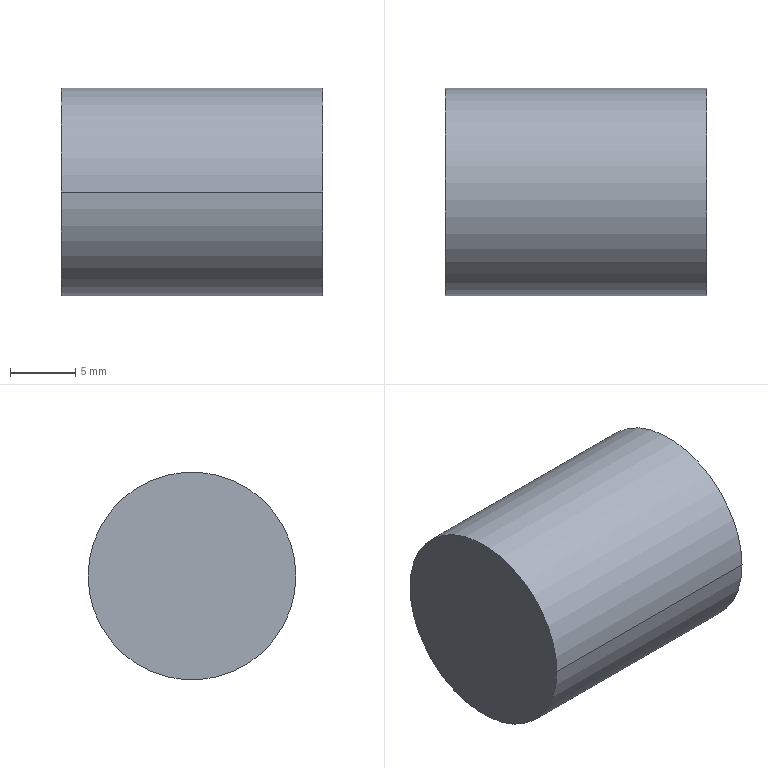Part | STEP file | 4-20.sldasm-Part-191 | 1 solid | 4 faces | box 20 x 15.87 x 15.87 mm | volume 3956 mm3 | cylinder 2 | plane 2 | commonest cylinder face diameters 15.87 x2
STEP:
#1=CARTESIAN_POINT('',(-213.37,-566.51,-38.));
#2=VERTEX_POINT('',#1);
#3=CARTESIAN_POINT('',(-213.37,-550.64,-38.));
#4=VERTEX_POINT('',#3);
#5=CARTESIAN_POINT('',(-213.37,-558.575,-38.));
#6=DIRECTION('',(1.,0.,0.));
#7=DIRECTION('',(0.,1.,0.));
#8=AXIS2_PLACEMENT_3D('',#5,#6,#7);
#9=CIRCLE('',#8,7.935);
#10=EDGE_CURVE('',#2,#4,#9,.T.);
#11=ORIENTED_EDGE('',*,*,#10,.T.);
#12=CARTESIAN_POINT('',(-193.37,-550.64,-38.));
#13=VERTEX_POINT('',#12);
#14=CARTESIAN_POINT('',(-203.37,-550.64,-38.));
#15=DIRECTION('',(1.,0.,0.));
#16=VECTOR('',#15,1000.);
#17=LINE('',#14,#16);
#18=EDGE_CURVE('',#4,#13,#17,.T.);
#19=ORIENTED_EDGE('',*,*,#18,.T.);
#20=CARTESIAN_POINT('',(-193.37,-566.51,-38.));
#21=VERTEX_POINT('',#20);
#22=CARTESIAN_POINT('',(-193.37,-558.575,-38.));
#23=DIRECTION('',(-1.,0.,0.));
#24=DIRECTION('',(0.,-1.,0.));
#25=AXIS2_PLACEMENT_3D('',#22,#23,#24);
#26=CIRCLE('',#25,7.935);
#27=EDGE_CURVE('',#13,#21,#26,.T.);
#28=ORIENTED_EDGE('',*,*,#27,.T.);
#29=CARTESIAN_POINT('',(-203.37,-566.51,-38.));
#30=DIRECTION('',(1.,0.,0.));
#31=VECTOR('',#30,1000.);
#32=LINE('',#29,#31);
#33=EDGE_CURVE('',#2,#21,#32,.T.);
#34=ORIENTED_EDGE('',*,*,#33,.F.);
#35=EDGE_LOOP('',(#11,#19,#28,#34));
#36=FACE_OUTER_BOUND('',#35,.T.);
#37=CARTESIAN_POINT('',(-203.37,-558.575,-38.));
#38=DIRECTION('',(1.,0.,0.));
#39=DIRECTION('',(0.,-1.,0.));
#40=AXIS2_PLACEMENT_3D('',#37,#38,#39);
#41=CYLINDRICAL_SURFACE('',#40,7.935);
#42=ADVANCED_FACE('',(#36),#41,.T.);
#43=CARTESIAN_POINT('',(-193.37,-558.575,-38.));
#44=DIRECTION('',(-1.,0.,0.));
#45=DIRECTION('',(0.,-1.,0.));
#46=AXIS2_PLACEMENT_3D('',#43,#44,#45);
#47=CIRCLE('',#46,7.935);
#48=EDGE_CURVE('',#21,#13,#47,.T.);
#49=ORIENTED_EDGE('',*,*,#48,.F.);
#50=ORIENTED_EDGE('',*,*,#27,.F.);
#51=EDGE_LOOP('',(#49,#50));
#52=FACE_OUTER_BOUND('',#51,.T.);
#53=CARTESIAN_POINT('',(-193.37,-558.575,-38.));
#54=DIRECTION('',(1.,0.,0.));
#55=DIRECTION('',(0.,-1.,0.));
#56=AXIS2_PLACEMENT_3D('',#53,#54,#55);
#57=PLANE('',#56);
#58=ADVANCED_FACE('',(#52),#57,.T.);
#59=ORIENTED_EDGE('',*,*,#10,.F.);
#60=CARTESIAN_POINT('',(-213.37,-558.575,-38.));
#61=DIRECTION('',(1.,0.,0.));
#62=DIRECTION('',(0.,1.,0.));
#63=AXIS2_PLACEMENT_3D('',#60,#61,#62);
#64=CIRCLE('',#63,7.935);
#65=EDGE_CURVE('',#4,#2,#64,.T.);
#66=ORIENTED_EDGE('',*,*,#65,.F.);
#67=EDGE_LOOP('',(#59,#66));
#68=FACE_OUTER_BOUND('',#67,.T.);
#69=CARTESIAN_POINT('',(-213.37,-558.575,-38.));
#70=DIRECTION('',(-1.,0.,0.));
#71=DIRECTION('',(0.,1.,0.));
#72=AXIS2_PLACEMENT_3D('',#69,#70,#71);
#73=PLANE('',#72);
#74=ADVANCED_FACE('',(#68),#73,.T.);
#75=ORIENTED_EDGE('',*,*,#18,.F.);
#76=ORIENTED_EDGE('',*,*,#65,.T.);
#77=ORIENTED_EDGE('',*,*,#33,.T.);
#78=ORIENTED_EDGE('',*,*,#48,.T.);
#79=EDGE_LOOP('',(#75,#76,#77,#78));
#80=FACE_OUTER_BOUND('',#79,.T.);
#81=CARTESIAN_POINT('',(-203.37,-558.575,-38.));
#82=DIRECTION('',(1.,0.,0.));
#83=DIRECTION('',(0.,-1.,0.));
#84=AXIS2_PLACEMENT_3D('',#81,#82,#83);
#85=CYLINDRICAL_SURFACE('',#84,7.935);
#86=ADVANCED_FACE('',(#80),#85,.T.);
#87=CLOSED_SHELL('',(#42,#58,#74,#86));
#88=MANIFOLD_SOLID_BREP('',#87);
#89=CARTESIAN_POINT('',(0.,0.,0.));
#90=DIRECTION('',(0.,0.,1.));
#91=DIRECTION('',(1.,0.,0.));
#92=AXIS2_PLACEMENT_3D('',#89,#90,#91);
#93=(LENGTH_UNIT()NAMED_UNIT(*)SI_UNIT(.MILLI.,.METRE.));
#94=UNCERTAINTY_MEASURE_WITH_UNIT(LENGTH_MEASURE(0.00001),#93,'','');
#95=(NAMED_UNIT(*)PLANE_ANGLE_UNIT()SI_UNIT($,.RADIAN.));
#96=(NAMED_UNIT(*)SI_UNIT($,.STERADIAN.)SOLID_ANGLE_UNIT());
#97=(GEOMETRIC_REPRESENTATION_CONTEXT(3)GLOBAL_UNCERTAINTY_ASSIGNED_CONTEXT((#94))GLOBAL_UNIT_ASSIGNED_CONTEXT((#93,#95,#96))REPRESENTATION_CONTEXT('',''));
#98=ADVANCED_BREP_SHAPE_REPRESENTATION('',(#88,#92),#97);